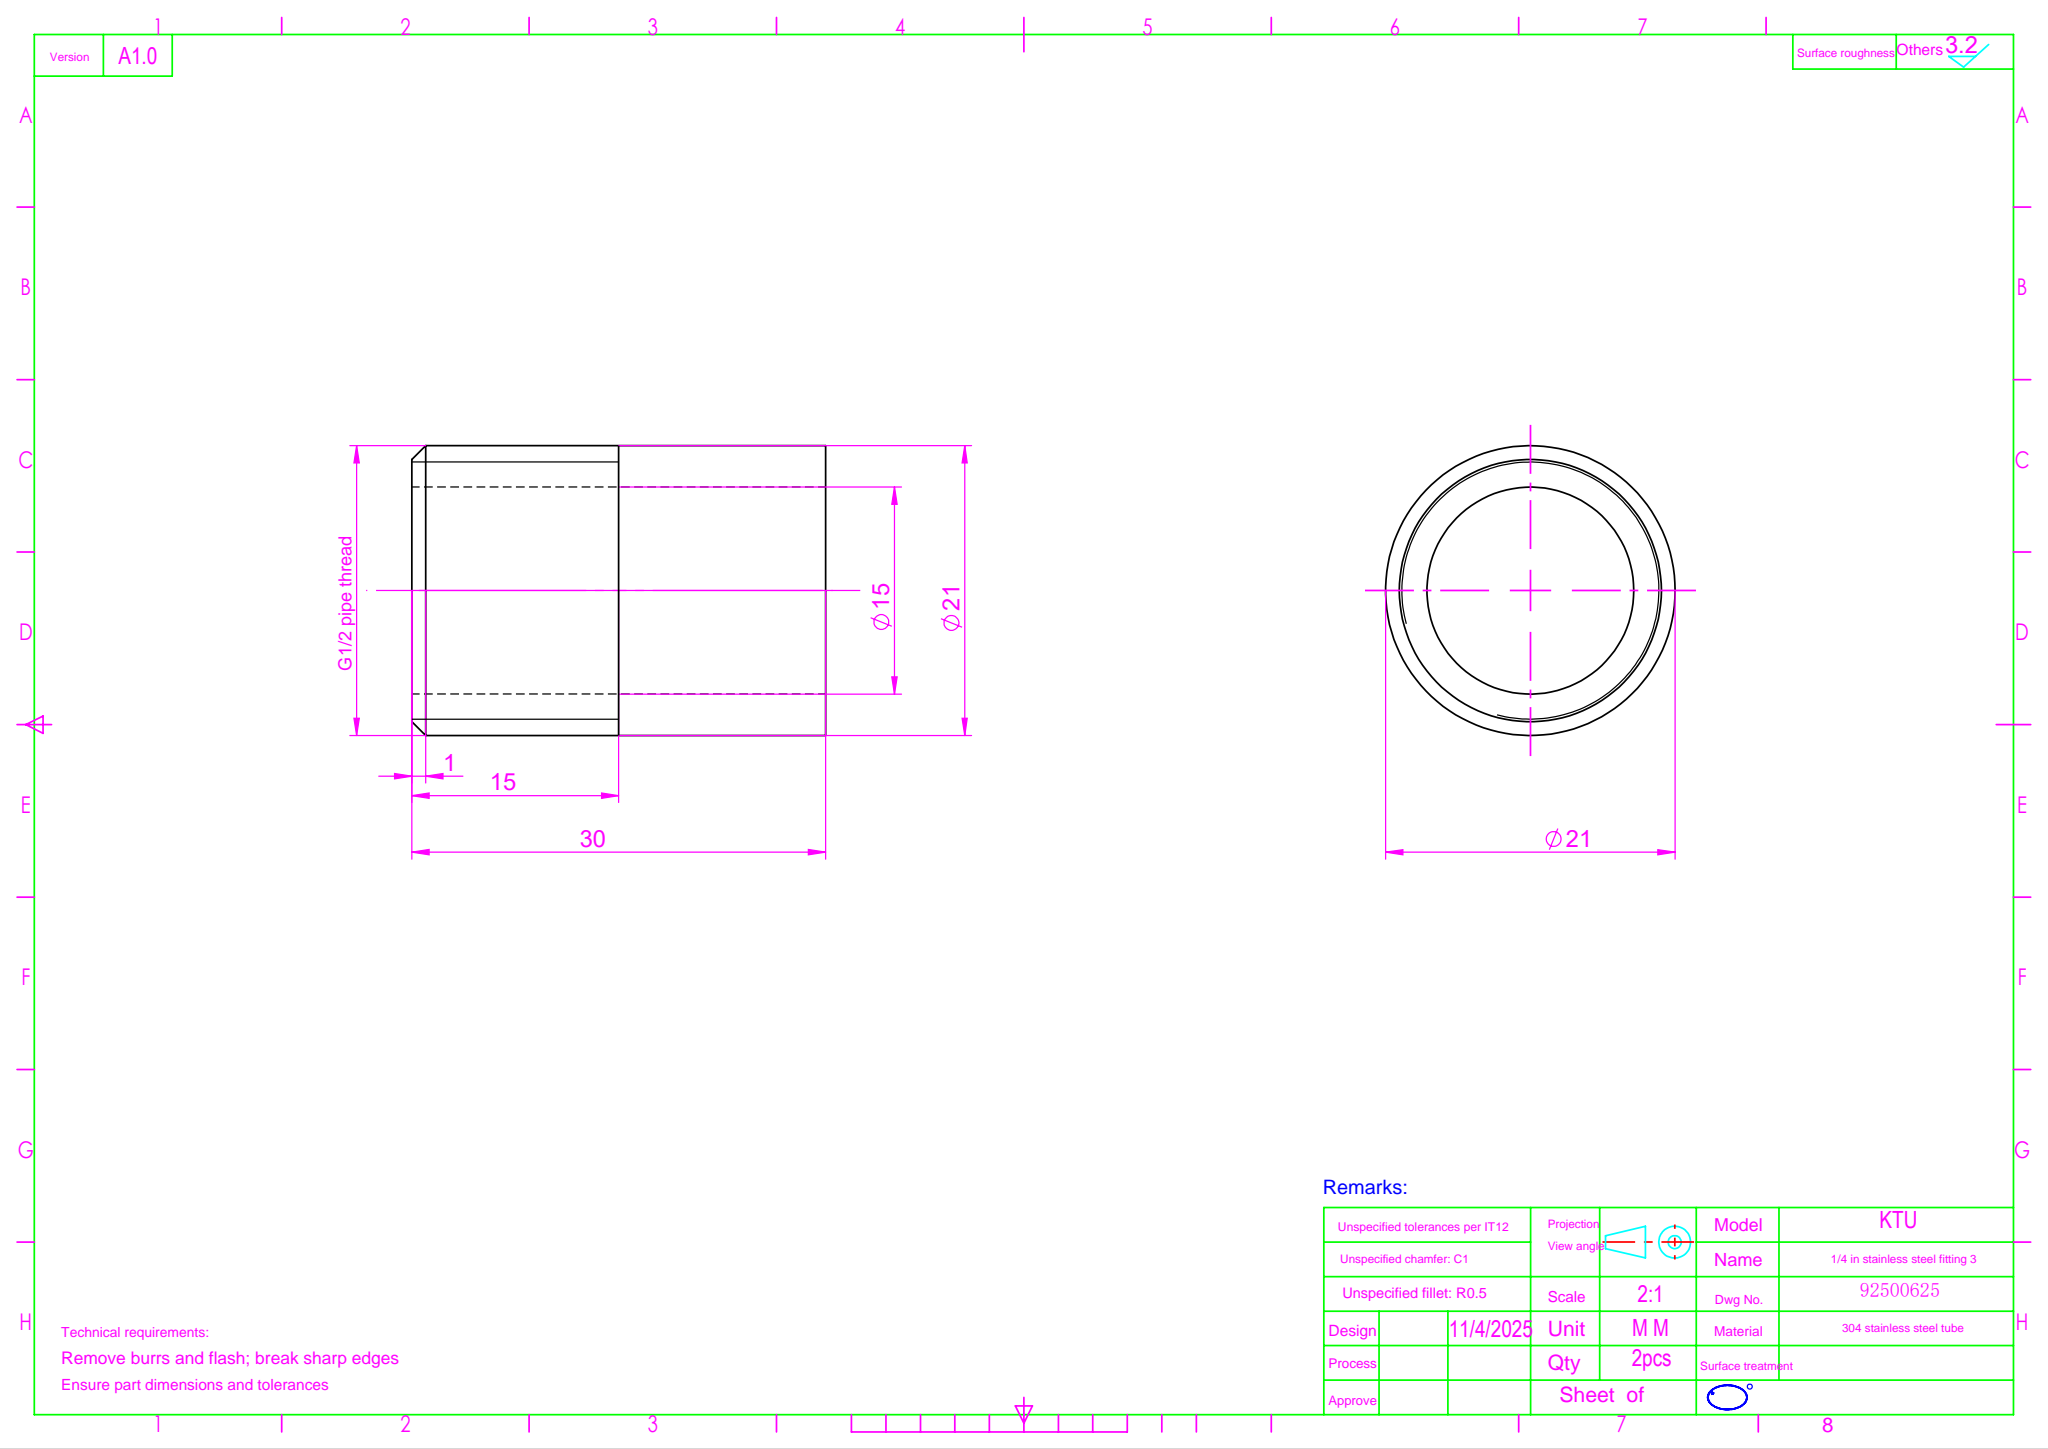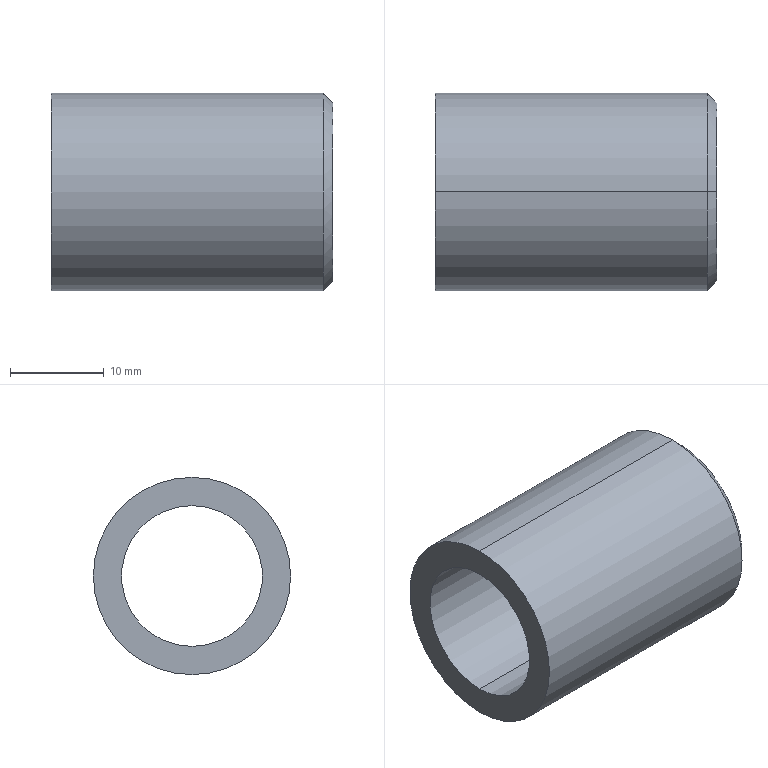Part | SolidWorks | features Chamfer 1, Extrusion 1 | 1 solid | 8 faces | box 30 x 21 x 21 mm | volume 5057 mm3 | cylinder 4 | cone 2 | plane 2 | commonest cylinder face diameters 15 x2 21 x2
STEP:
#1=CARTESIAN_POINT('',(15.,0.,-9.5));
#2=VERTEX_POINT('',#1);
#3=CARTESIAN_POINT('',(15.,0.,9.5));
#4=VERTEX_POINT('',#3);
#5=CARTESIAN_POINT('',(15.,0.,0.));
#6=DIRECTION('',(1.,0.,0.));
#7=DIRECTION('',(0.,0.,-1.));
#8=AXIS2_PLACEMENT_3D('',#5,#6,#7);
#9=CIRCLE('',#8,9.5);
#10=EDGE_CURVE('',#2,#4,#9,.T.);
#11=ORIENTED_EDGE('',*,*,#10,.F.);
#12=CARTESIAN_POINT('',(14.,0.,-10.5));
#13=VERTEX_POINT('',#12);
#14=CARTESIAN_POINT('',(15.,0.,-9.5));
#15=DIRECTION('',(-0.7071,0.,-0.7071));
#16=VECTOR('',#15,1000.);
#17=LINE('',#14,#16);
#18=EDGE_CURVE('',#2,#13,#17,.T.);
#19=ORIENTED_EDGE('',*,*,#18,.T.);
#20=CARTESIAN_POINT('',(14.,0.,10.5));
#21=VERTEX_POINT('',#20);
#22=CARTESIAN_POINT('',(14.,0.,0.));
#23=DIRECTION('',(-1.,0.,0.));
#24=DIRECTION('',(0.,0.,-1.));
#25=AXIS2_PLACEMENT_3D('',#22,#23,#24);
#26=CIRCLE('',#25,10.5);
#27=EDGE_CURVE('',#21,#13,#26,.T.);
#28=ORIENTED_EDGE('',*,*,#27,.F.);
#29=CARTESIAN_POINT('',(15.,0.,9.5));
#30=DIRECTION('',(-0.7071,0.,0.7071));
#31=VECTOR('',#30,1000.);
#32=LINE('',#29,#31);
#33=EDGE_CURVE('',#4,#21,#32,.T.);
#34=ORIENTED_EDGE('',*,*,#33,.F.);
#35=EDGE_LOOP('',(#11,#19,#28,#34));
#36=FACE_OUTER_BOUND('',#35,.T.);
#37=CARTESIAN_POINT('',(15.,0.,0.));
#38=DIRECTION('',(-1.,0.,0.));
#39=DIRECTION('',(0.,0.,1.));
#40=AXIS2_PLACEMENT_3D('',#37,#38,#39);
#41=CONICAL_SURFACE('',#40,9.5,0.7854);
#42=ADVANCED_FACE('',(#36),#41,.T.);
#43=CARTESIAN_POINT('',(15.,0.,7.5));
#44=VERTEX_POINT('',#43);
#45=CARTESIAN_POINT('',(15.,0.,-7.5));
#46=VERTEX_POINT('',#45);
#47=CARTESIAN_POINT('',(15.,0.,0.));
#48=DIRECTION('',(1.,0.,0.));
#49=DIRECTION('',(0.,0.,-1.));
#50=AXIS2_PLACEMENT_3D('',#47,#48,#49);
#51=CIRCLE('',#50,7.5);
#52=EDGE_CURVE('',#44,#46,#51,.T.);
#53=ORIENTED_EDGE('',*,*,#52,.T.);
#54=CARTESIAN_POINT('',(-15.,0.,-7.5));
#55=VERTEX_POINT('',#54);
#56=CARTESIAN_POINT('',(15.,0.,-7.5));
#57=DIRECTION('',(-1.,0.,0.));
#58=VECTOR('',#57,1000.);
#59=LINE('',#56,#58);
#60=EDGE_CURVE('',#46,#55,#59,.T.);
#61=ORIENTED_EDGE('',*,*,#60,.T.);
#62=CARTESIAN_POINT('',(-15.,0.,7.5));
#63=VERTEX_POINT('',#62);
#64=CARTESIAN_POINT('',(-15.,0.,0.));
#65=DIRECTION('',(1.,0.,0.));
#66=DIRECTION('',(0.,0.,-1.));
#67=AXIS2_PLACEMENT_3D('',#64,#65,#66);
#68=CIRCLE('',#67,7.5);
#69=EDGE_CURVE('',#63,#55,#68,.T.);
#70=ORIENTED_EDGE('',*,*,#69,.F.);
#71=CARTESIAN_POINT('',(15.,0.,7.5));
#72=DIRECTION('',(-1.,0.,0.));
#73=VECTOR('',#72,1000.);
#74=LINE('',#71,#73);
#75=EDGE_CURVE('',#44,#63,#74,.T.);
#76=ORIENTED_EDGE('',*,*,#75,.F.);
#77=EDGE_LOOP('',(#53,#61,#70,#76));
#78=FACE_OUTER_BOUND('',#77,.T.);
#79=CARTESIAN_POINT('',(15.,0.,0.));
#80=DIRECTION('',(-1.,0.,0.));
#81=DIRECTION('',(0.,0.,1.));
#82=AXIS2_PLACEMENT_3D('',#79,#80,#81);
#83=CYLINDRICAL_SURFACE('',#82,7.5);
#84=ADVANCED_FACE('',(#78),#83,.F.);
#85=ORIENTED_EDGE('',*,*,#27,.T.);
#86=CARTESIAN_POINT('',(-15.,0.,-10.5));
#87=VERTEX_POINT('',#86);
#88=CARTESIAN_POINT('',(15.,0.,-10.5));
#89=DIRECTION('',(-1.,0.,0.));
#90=VECTOR('',#89,1000.);
#91=LINE('',#88,#90);
#92=EDGE_CURVE('',#13,#87,#91,.T.);
#93=ORIENTED_EDGE('',*,*,#92,.T.);
#94=CARTESIAN_POINT('',(-15.,0.,10.5));
#95=VERTEX_POINT('',#94);
#96=CARTESIAN_POINT('',(-15.,0.,0.));
#97=DIRECTION('',(1.,0.,0.));
#98=DIRECTION('',(0.,0.,-1.));
#99=AXIS2_PLACEMENT_3D('',#96,#97,#98);
#100=CIRCLE('',#99,10.5);
#101=EDGE_CURVE('',#87,#95,#100,.T.);
#102=ORIENTED_EDGE('',*,*,#101,.T.);
#103=CARTESIAN_POINT('',(15.,0.,10.5));
#104=DIRECTION('',(-1.,0.,0.));
#105=VECTOR('',#104,1000.);
#106=LINE('',#103,#105);
#107=EDGE_CURVE('',#21,#95,#106,.T.);
#108=ORIENTED_EDGE('',*,*,#107,.F.);
#109=EDGE_LOOP('',(#85,#93,#102,#108));
#110=FACE_OUTER_BOUND('',#109,.T.);
#111=CARTESIAN_POINT('',(15.,0.,0.));
#112=DIRECTION('',(-1.,0.,0.));
#113=DIRECTION('',(0.,0.,1.));
#114=AXIS2_PLACEMENT_3D('',#111,#112,#113);
#115=CYLINDRICAL_SURFACE('',#114,10.5);
#116=ADVANCED_FACE('',(#110),#115,.T.);
#117=CARTESIAN_POINT('',(15.,0.,0.));
#118=DIRECTION('',(1.,0.,0.));
#119=DIRECTION('',(0.,0.,-1.));
#120=AXIS2_PLACEMENT_3D('',#117,#118,#119);
#121=CIRCLE('',#120,9.5);
#122=EDGE_CURVE('',#4,#2,#121,.T.);
#123=ORIENTED_EDGE('',*,*,#122,.T.);
#124=ORIENTED_EDGE('',*,*,#10,.T.);
#125=EDGE_LOOP('',(#123,#124));
#126=FACE_OUTER_BOUND('',#125,.T.);
#127=ORIENTED_EDGE('',*,*,#52,.F.);
#128=CARTESIAN_POINT('',(15.,0.,0.));
#129=DIRECTION('',(1.,0.,0.));
#130=DIRECTION('',(0.,0.,-1.));
#131=AXIS2_PLACEMENT_3D('',#128,#129,#130);
#132=CIRCLE('',#131,7.5);
#133=EDGE_CURVE('',#46,#44,#132,.T.);
#134=ORIENTED_EDGE('',*,*,#133,.F.);
#135=EDGE_LOOP('',(#127,#134));
#136=FACE_BOUND('',#135,.T.);
#137=CARTESIAN_POINT('',(15.,0.,0.));
#138=DIRECTION('',(1.,0.,0.));
#139=DIRECTION('',(0.,0.,-1.));
#140=AXIS2_PLACEMENT_3D('',#137,#138,#139);
#141=PLANE('',#140);
#142=ADVANCED_FACE('',(#126,#136),#141,.T.);
#143=CARTESIAN_POINT('',(-15.,0.,0.));
#144=DIRECTION('',(1.,0.,0.));
#145=DIRECTION('',(0.,0.,-1.));
#146=AXIS2_PLACEMENT_3D('',#143,#144,#145);
#147=CIRCLE('',#146,10.5);
#148=EDGE_CURVE('',#95,#87,#147,.T.);
#149=ORIENTED_EDGE('',*,*,#148,.F.);
#150=ORIENTED_EDGE('',*,*,#101,.F.);
#151=EDGE_LOOP('',(#149,#150));
#152=FACE_OUTER_BOUND('',#151,.T.);
#153=ORIENTED_EDGE('',*,*,#69,.T.);
#154=CARTESIAN_POINT('',(-15.,0.,0.));
#155=DIRECTION('',(1.,0.,0.));
#156=DIRECTION('',(0.,0.,-1.));
#157=AXIS2_PLACEMENT_3D('',#154,#155,#156);
#158=CIRCLE('',#157,7.5);
#159=EDGE_CURVE('',#55,#63,#158,.T.);
#160=ORIENTED_EDGE('',*,*,#159,.T.);
#161=EDGE_LOOP('',(#153,#160));
#162=FACE_BOUND('',#161,.T.);
#163=CARTESIAN_POINT('',(-15.,0.,0.));
#164=DIRECTION('',(1.,0.,0.));
#165=DIRECTION('',(0.,0.,-1.));
#166=AXIS2_PLACEMENT_3D('',#163,#164,#165);
#167=PLANE('',#166);
#168=ADVANCED_FACE('',(#152,#162),#167,.F.);
#169=ORIENTED_EDGE('',*,*,#92,.F.);
#170=CARTESIAN_POINT('',(14.,0.,0.));
#171=DIRECTION('',(-1.,0.,0.));
#172=DIRECTION('',(0.,0.,-1.));
#173=AXIS2_PLACEMENT_3D('',#170,#171,#172);
#174=CIRCLE('',#173,10.5);
#175=EDGE_CURVE('',#13,#21,#174,.T.);
#176=ORIENTED_EDGE('',*,*,#175,.T.);
#177=ORIENTED_EDGE('',*,*,#107,.T.);
#178=ORIENTED_EDGE('',*,*,#148,.T.);
#179=EDGE_LOOP('',(#169,#176,#177,#178));
#180=FACE_OUTER_BOUND('',#179,.T.);
#181=CARTESIAN_POINT('',(15.,0.,0.));
#182=DIRECTION('',(-1.,0.,0.));
#183=DIRECTION('',(0.,0.,1.));
#184=AXIS2_PLACEMENT_3D('',#181,#182,#183);
#185=CYLINDRICAL_SURFACE('',#184,10.5);
#186=ADVANCED_FACE('',(#180),#185,.T.);
#187=ORIENTED_EDGE('',*,*,#60,.F.);
#188=ORIENTED_EDGE('',*,*,#133,.T.);
#189=ORIENTED_EDGE('',*,*,#75,.T.);
#190=ORIENTED_EDGE('',*,*,#159,.F.);
#191=EDGE_LOOP('',(#187,#188,#189,#190));
#192=FACE_OUTER_BOUND('',#191,.T.);
#193=CARTESIAN_POINT('',(15.,0.,0.));
#194=DIRECTION('',(-1.,0.,0.));
#195=DIRECTION('',(0.,0.,1.));
#196=AXIS2_PLACEMENT_3D('',#193,#194,#195);
#197=CYLINDRICAL_SURFACE('',#196,7.5);
#198=ADVANCED_FACE('',(#192),#197,.F.);
#199=ORIENTED_EDGE('',*,*,#18,.F.);
#200=ORIENTED_EDGE('',*,*,#122,.F.);
#201=ORIENTED_EDGE('',*,*,#33,.T.);
#202=ORIENTED_EDGE('',*,*,#175,.F.);
#203=EDGE_LOOP('',(#199,#200,#201,#202));
#204=FACE_OUTER_BOUND('',#203,.T.);
#205=CARTESIAN_POINT('',(15.,0.,0.));
#206=DIRECTION('',(-1.,0.,0.));
#207=DIRECTION('',(0.,0.,1.));
#208=AXIS2_PLACEMENT_3D('',#205,#206,#207);
#209=CONICAL_SURFACE('',#208,9.5,0.7854);
#210=ADVANCED_FACE('',(#204),#209,.T.);
#211=CLOSED_SHELL('',(#42,#84,#116,#142,#168,#186,#198,#210));
#212=MANIFOLD_SOLID_BREP('',#211);
#213=CARTESIAN_POINT('',(0.,0.,0.));
#214=DIRECTION('',(0.,0.,1.));
#215=DIRECTION('',(1.,0.,0.));
#216=AXIS2_PLACEMENT_3D('',#213,#214,#215);
#217=(LENGTH_UNIT()NAMED_UNIT(*)SI_UNIT(.MILLI.,.METRE.));
#218=UNCERTAINTY_MEASURE_WITH_UNIT(LENGTH_MEASURE(0.00001),#217,'','');
#219=(NAMED_UNIT(*)PLANE_ANGLE_UNIT()SI_UNIT($,.RADIAN.));
#220=(NAMED_UNIT(*)SI_UNIT($,.STERADIAN.)SOLID_ANGLE_UNIT());
#221=(GEOMETRIC_REPRESENTATION_CONTEXT(3)GLOBAL_UNCERTAINTY_ASSIGNED_CONTEXT((#218))GLOBAL_UNIT_ASSIGNED_CONTEXT((#217,#219,#220))REPRESENTATION_CONTEXT('',''));
#222=ADVANCED_BREP_SHAPE_REPRESENTATION('',(#212,#216),#221);